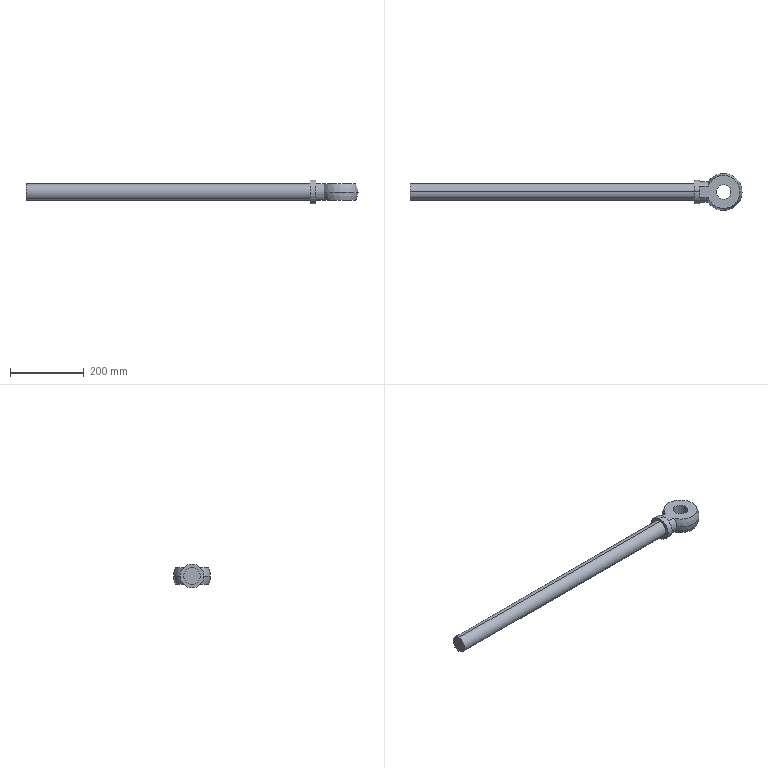Part | SolidWorks | features ICE 2, Revolution 1 | 1 solid | 15 faces | box 900 x 100 x 65 mm | volume 1587827 mm3 | cylinder 8 | plane 5 | sphere 2 | commonest cylinder face diameters 40 x2 45 x2 55 x2 65 x2
STEP:
#1=CARTESIAN_POINT('',(80.,0.,22.5));
#2=VERTEX_POINT('',#1);
#3=CARTESIAN_POINT('',(120.,0.,22.5));
#4=VERTEX_POINT('',#3);
#5=CARTESIAN_POINT('',(100.,0.,22.5));
#6=DIRECTION('',(0.,0.,1.));
#7=DIRECTION('',(1.,0.,0.));
#8=AXIS2_PLACEMENT_3D('',#5,#6,#7);
#9=CIRCLE('',#8,20.);
#10=EDGE_CURVE('',#2,#4,#9,.T.);
#11=ORIENTED_EDGE('',*,*,#10,.T.);
#12=CARTESIAN_POINT('',(120.,0.,-22.5));
#13=VERTEX_POINT('',#12);
#14=CARTESIAN_POINT('',(120.,0.,32.5));
#15=DIRECTION('',(0.,0.,-1.));
#16=VECTOR('',#15,1000.);
#17=LINE('',#14,#16);
#18=EDGE_CURVE('',#4,#13,#17,.T.);
#19=ORIENTED_EDGE('',*,*,#18,.T.);
#20=CARTESIAN_POINT('',(80.,0.,-22.5));
#21=VERTEX_POINT('',#20);
#22=CARTESIAN_POINT('',(100.,0.,-22.5));
#23=DIRECTION('',(0.,0.,-1.));
#24=DIRECTION('',(-1.,0.,0.));
#25=AXIS2_PLACEMENT_3D('',#22,#23,#24);
#26=CIRCLE('',#25,20.);
#27=EDGE_CURVE('',#13,#21,#26,.T.);
#28=ORIENTED_EDGE('',*,*,#27,.T.);
#29=CARTESIAN_POINT('',(80.,0.,32.5));
#30=DIRECTION('',(0.,0.,-1.));
#31=VECTOR('',#30,1000.);
#32=LINE('',#29,#31);
#33=EDGE_CURVE('',#2,#21,#32,.T.);
#34=ORIENTED_EDGE('',*,*,#33,.F.);
#35=EDGE_LOOP('',(#11,#19,#28,#34));
#36=FACE_OUTER_BOUND('',#35,.T.);
#37=CARTESIAN_POINT('',(100.,0.,32.5));
#38=DIRECTION('',(0.,0.,-1.));
#39=DIRECTION('',(-1.,0.,0.));
#40=AXIS2_PLACEMENT_3D('',#37,#38,#39);
#41=CYLINDRICAL_SURFACE('',#40,20.);
#42=ADVANCED_FACE('',(#36),#41,.F.);
#43=CARTESIAN_POINT('',(20.,0.,22.5));
#44=VERTEX_POINT('',#43);
#45=CARTESIAN_POINT('',(20.,0.,-22.5));
#46=VERTEX_POINT('',#45);
#47=CARTESIAN_POINT('',(20.,0.,0.));
#48=DIRECTION('',(-1.,0.,0.));
#49=DIRECTION('',(0.,0.,1.));
#50=AXIS2_PLACEMENT_3D('',#47,#48,#49);
#51=CIRCLE('',#50,22.5);
#52=EDGE_CURVE('',#44,#46,#51,.T.);
#53=ORIENTED_EDGE('',*,*,#52,.T.);
#54=CARTESIAN_POINT('',(-750.,0.,-22.5));
#55=VERTEX_POINT('',#54);
#56=CARTESIAN_POINT('',(-750.,0.,-22.5));
#57=DIRECTION('',(-1.,0.,0.));
#58=VECTOR('',#57,1000.);
#59=LINE('',#56,#58);
#60=EDGE_CURVE('',#46,#55,#59,.T.);
#61=ORIENTED_EDGE('',*,*,#60,.T.);
#62=CARTESIAN_POINT('',(-750.,0.,22.5));
#63=VERTEX_POINT('',#62);
#64=CARTESIAN_POINT('',(-750.,0.,0.));
#65=DIRECTION('',(-1.,0.,0.));
#66=DIRECTION('',(0.,0.,1.));
#67=AXIS2_PLACEMENT_3D('',#64,#65,#66);
#68=CIRCLE('',#67,22.5);
#69=EDGE_CURVE('',#63,#55,#68,.T.);
#70=ORIENTED_EDGE('',*,*,#69,.F.);
#71=CARTESIAN_POINT('',(-750.,0.,22.5));
#72=DIRECTION('',(-1.,0.,0.));
#73=VECTOR('',#72,1000.);
#74=LINE('',#71,#73);
#75=EDGE_CURVE('',#44,#63,#74,.T.);
#76=ORIENTED_EDGE('',*,*,#75,.F.);
#77=EDGE_LOOP('',(#53,#61,#70,#76));
#78=FACE_OUTER_BOUND('',#77,.T.);
#79=CARTESIAN_POINT('',(-750.,0.,0.));
#80=DIRECTION('',(-1.,0.,0.));
#81=DIRECTION('',(0.,0.,1.));
#82=AXIS2_PLACEMENT_3D('',#79,#80,#81);
#83=CYLINDRICAL_SURFACE('',#82,22.5);
#84=ADVANCED_FACE('',(#78),#83,.T.);
#85=CARTESIAN_POINT('',(35.,0.,32.5));
#86=VERTEX_POINT('',#85);
#87=CARTESIAN_POINT('',(35.,0.,-32.5));
#88=VERTEX_POINT('',#87);
#89=CARTESIAN_POINT('',(35.,0.,0.));
#90=DIRECTION('',(-1.,0.,0.));
#91=DIRECTION('',(0.,0.,1.));
#92=AXIS2_PLACEMENT_3D('',#89,#90,#91);
#93=CIRCLE('',#92,32.5);
#94=EDGE_CURVE('',#86,#88,#93,.T.);
#95=ORIENTED_EDGE('',*,*,#94,.T.);
#96=CARTESIAN_POINT('',(20.,0.,-32.5));
#97=VERTEX_POINT('',#96);
#98=CARTESIAN_POINT('',(-750.,0.,-32.5));
#99=DIRECTION('',(-1.,0.,0.));
#100=VECTOR('',#99,1000.);
#101=LINE('',#98,#100);
#102=EDGE_CURVE('',#88,#97,#101,.T.);
#103=ORIENTED_EDGE('',*,*,#102,.T.);
#104=CARTESIAN_POINT('',(20.,0.,32.5));
#105=VERTEX_POINT('',#104);
#106=CARTESIAN_POINT('',(20.,0.,0.));
#107=DIRECTION('',(-1.,0.,0.));
#108=DIRECTION('',(0.,0.,1.));
#109=AXIS2_PLACEMENT_3D('',#106,#107,#108);
#110=CIRCLE('',#109,32.5);
#111=EDGE_CURVE('',#105,#97,#110,.T.);
#112=ORIENTED_EDGE('',*,*,#111,.F.);
#113=CARTESIAN_POINT('',(-750.,0.,32.5));
#114=DIRECTION('',(-1.,0.,0.));
#115=VECTOR('',#114,1000.);
#116=LINE('',#113,#115);
#117=EDGE_CURVE('',#86,#105,#116,.T.);
#118=ORIENTED_EDGE('',*,*,#117,.F.);
#119=EDGE_LOOP('',(#95,#103,#112,#118));
#120=FACE_OUTER_BOUND('',#119,.T.);
#121=CARTESIAN_POINT('',(-750.,0.,0.));
#122=DIRECTION('',(-1.,0.,0.));
#123=DIRECTION('',(0.,0.,1.));
#124=AXIS2_PLACEMENT_3D('',#121,#122,#123);
#125=CYLINDRICAL_SURFACE('',#124,32.5);
#126=ADVANCED_FACE('',(#120),#125,.T.);
#127=CARTESIAN_POINT('',(150.,0.,0.));
#128=VERTEX_POINT('',#127);
#129=CARTESIAN_POINT('',(58.242,27.5,0.));
#130=VERTEX_POINT('',#129);
#131=CARTESIAN_POINT('',(100.,0.,0.));
#132=DIRECTION('',(0.,0.,1.));
#133=DIRECTION('',(1.,0.,0.));
#134=AXIS2_PLACEMENT_3D('',#131,#132,#133);
#135=CIRCLE('',#134,50.);
#136=EDGE_CURVE('',#128,#130,#135,.T.);
#137=ORIENTED_EDGE('',*,*,#136,.F.);
#138=CARTESIAN_POINT('',(58.242,-27.5,0.));
#139=VERTEX_POINT('',#138);
#140=CARTESIAN_POINT('',(100.,0.,0.));
#141=DIRECTION('',(0.,0.,-1.));
#142=DIRECTION('',(0.,1.,0.));
#143=AXIS2_PLACEMENT_3D('',#140,#141,#142);
#144=CIRCLE('',#143,50.);
#145=EDGE_CURVE('',#128,#139,#144,.T.);
#146=ORIENTED_EDGE('',*,*,#145,.T.);
#147=CARTESIAN_POINT('',(58.242,-15.811,-22.5));
#148=VERTEX_POINT('',#147);
#149=CARTESIAN_POINT('',(58.242,0.,0.));
#150=DIRECTION('',(-1.,0.,0.));
#151=DIRECTION('',(0.,0.,1.));
#152=AXIS2_PLACEMENT_3D('',#149,#150,#151);
#153=CIRCLE('',#152,27.5);
#154=EDGE_CURVE('',#148,#139,#153,.T.);
#155=ORIENTED_EDGE('',*,*,#154,.F.);
#156=CARTESIAN_POINT('',(58.242,15.811,-22.5));
#157=VERTEX_POINT('',#156);
#158=CARTESIAN_POINT('',(100.,0.,-22.5));
#159=DIRECTION('',(0.,0.,-1.));
#160=DIRECTION('',(-1.,0.,0.));
#161=AXIS2_PLACEMENT_3D('',#158,#159,#160);
#162=CIRCLE('',#161,44.651);
#163=EDGE_CURVE('',#157,#148,#162,.T.);
#164=ORIENTED_EDGE('',*,*,#163,.F.);
#165=CARTESIAN_POINT('',(58.242,0.,0.));
#166=DIRECTION('',(-1.,0.,0.));
#167=DIRECTION('',(0.,0.,1.));
#168=AXIS2_PLACEMENT_3D('',#165,#166,#167);
#169=CIRCLE('',#168,27.5);
#170=EDGE_CURVE('',#130,#157,#169,.T.);
#171=ORIENTED_EDGE('',*,*,#170,.F.);
#172=EDGE_LOOP('',(#137,#146,#155,#164,#171));
#173=FACE_OUTER_BOUND('',#172,.T.);
#174=CARTESIAN_POINT('',(100.,0.,0.));
#175=DIRECTION('',(0.,0.,-1.));
#176=DIRECTION('',(0.,1.,0.));
#177=AXIS2_PLACEMENT_3D('',#174,#175,#176);
#178=SPHERICAL_SURFACE('',#177,50.);
#179=ADVANCED_FACE('',(#173),#178,.T.);
#180=ORIENTED_EDGE('',*,*,#145,.F.);
#181=ORIENTED_EDGE('',*,*,#136,.T.);
#182=CARTESIAN_POINT('',(58.242,15.811,22.5));
#183=VERTEX_POINT('',#182);
#184=CARTESIAN_POINT('',(58.242,0.,0.));
#185=DIRECTION('',(-1.,0.,0.));
#186=DIRECTION('',(0.,0.,1.));
#187=AXIS2_PLACEMENT_3D('',#184,#185,#186);
#188=CIRCLE('',#187,27.5);
#189=EDGE_CURVE('',#183,#130,#188,.T.);
#190=ORIENTED_EDGE('',*,*,#189,.F.);
#191=CARTESIAN_POINT('',(58.242,-15.811,22.5));
#192=VERTEX_POINT('',#191);
#193=CARTESIAN_POINT('',(100.,0.,22.5));
#194=DIRECTION('',(0.,0.,1.));
#195=DIRECTION('',(1.,0.,0.));
#196=AXIS2_PLACEMENT_3D('',#193,#194,#195);
#197=CIRCLE('',#196,44.651);
#198=EDGE_CURVE('',#192,#183,#197,.T.);
#199=ORIENTED_EDGE('',*,*,#198,.F.);
#200=CARTESIAN_POINT('',(58.242,0.,0.));
#201=DIRECTION('',(-1.,0.,0.));
#202=DIRECTION('',(0.,0.,1.));
#203=AXIS2_PLACEMENT_3D('',#200,#201,#202);
#204=CIRCLE('',#203,27.5);
#205=EDGE_CURVE('',#139,#192,#204,.T.);
#206=ORIENTED_EDGE('',*,*,#205,.F.);
#207=EDGE_LOOP('',(#180,#181,#190,#199,#206));
#208=FACE_OUTER_BOUND('',#207,.T.);
#209=CARTESIAN_POINT('',(100.,0.,0.));
#210=DIRECTION('',(0.,0.,-1.));
#211=DIRECTION('',(0.,1.,0.));
#212=AXIS2_PLACEMENT_3D('',#209,#210,#211);
#213=SPHERICAL_SURFACE('',#212,50.);
#214=ADVANCED_FACE('',(#208),#213,.T.);
#215=CARTESIAN_POINT('',(35.,15.811,22.5));
#216=VERTEX_POINT('',#215);
#217=CARTESIAN_POINT('',(-750.,15.811,22.5));
#218=DIRECTION('',(-1.,0.,0.));
#219=VECTOR('',#218,1000.);
#220=LINE('',#217,#219);
#221=EDGE_CURVE('',#183,#216,#220,.T.);
#222=ORIENTED_EDGE('',*,*,#221,.F.);
#223=ORIENTED_EDGE('',*,*,#189,.T.);
#224=ORIENTED_EDGE('',*,*,#170,.T.);
#225=CARTESIAN_POINT('',(35.,15.811,-22.5));
#226=VERTEX_POINT('',#225);
#227=CARTESIAN_POINT('',(-750.,15.811,-22.5));
#228=DIRECTION('',(1.,0.,0.));
#229=VECTOR('',#228,1000.);
#230=LINE('',#227,#229);
#231=EDGE_CURVE('',#226,#157,#230,.T.);
#232=ORIENTED_EDGE('',*,*,#231,.F.);
#233=CARTESIAN_POINT('',(35.,0.,0.));
#234=DIRECTION('',(-1.,0.,0.));
#235=DIRECTION('',(0.,0.,1.));
#236=AXIS2_PLACEMENT_3D('',#233,#234,#235);
#237=CIRCLE('',#236,27.5);
#238=EDGE_CURVE('',#216,#226,#237,.T.);
#239=ORIENTED_EDGE('',*,*,#238,.F.);
#240=EDGE_LOOP('',(#222,#223,#224,#232,#239));
#241=FACE_OUTER_BOUND('',#240,.T.);
#242=CARTESIAN_POINT('',(-750.,0.,0.));
#243=DIRECTION('',(-1.,0.,0.));
#244=DIRECTION('',(0.,0.,1.));
#245=AXIS2_PLACEMENT_3D('',#242,#243,#244);
#246=CYLINDRICAL_SURFACE('',#245,27.5);
#247=ADVANCED_FACE('',(#241),#246,.T.);
#248=CARTESIAN_POINT('',(35.,-15.811,22.5));
#249=VERTEX_POINT('',#248);
#250=CARTESIAN_POINT('',(-750.,-15.811,22.5));
#251=DIRECTION('',(1.,0.,0.));
#252=VECTOR('',#251,1000.);
#253=LINE('',#250,#252);
#254=EDGE_CURVE('',#249,#192,#253,.T.);
#255=ORIENTED_EDGE('',*,*,#254,.F.);
#256=CARTESIAN_POINT('',(35.,-15.811,-22.5));
#257=VERTEX_POINT('',#256);
#258=CARTESIAN_POINT('',(35.,0.,0.));
#259=DIRECTION('',(-1.,0.,0.));
#260=DIRECTION('',(0.,0.,1.));
#261=AXIS2_PLACEMENT_3D('',#258,#259,#260);
#262=CIRCLE('',#261,27.5);
#263=EDGE_CURVE('',#257,#249,#262,.T.);
#264=ORIENTED_EDGE('',*,*,#263,.F.);
#265=CARTESIAN_POINT('',(-750.,-15.811,-22.5));
#266=DIRECTION('',(-1.,0.,0.));
#267=VECTOR('',#266,1000.);
#268=LINE('',#265,#267);
#269=EDGE_CURVE('',#148,#257,#268,.T.);
#270=ORIENTED_EDGE('',*,*,#269,.F.);
#271=ORIENTED_EDGE('',*,*,#154,.T.);
#272=ORIENTED_EDGE('',*,*,#205,.T.);
#273=EDGE_LOOP('',(#255,#264,#270,#271,#272));
#274=FACE_OUTER_BOUND('',#273,.T.);
#275=CARTESIAN_POINT('',(-750.,0.,0.));
#276=DIRECTION('',(-1.,0.,0.));
#277=DIRECTION('',(0.,0.,1.));
#278=AXIS2_PLACEMENT_3D('',#275,#276,#277);
#279=CYLINDRICAL_SURFACE('',#278,27.5);
#280=ADVANCED_FACE('',(#274),#279,.T.);
#281=ORIENTED_EDGE('',*,*,#263,.T.);
#282=CARTESIAN_POINT('',(35.,68.387,22.5));
#283=DIRECTION('',(0.,1.,0.));
#284=VECTOR('',#283,1000.);
#285=LINE('',#282,#284);
#286=EDGE_CURVE('',#249,#216,#285,.T.);
#287=ORIENTED_EDGE('',*,*,#286,.T.);
#288=ORIENTED_EDGE('',*,*,#238,.T.);
#289=CARTESIAN_POINT('',(35.,68.387,-22.5));
#290=DIRECTION('',(0.,-1.,0.));
#291=VECTOR('',#290,1000.);
#292=LINE('',#289,#291);
#293=EDGE_CURVE('',#226,#257,#292,.T.);
#294=ORIENTED_EDGE('',*,*,#293,.T.);
#295=EDGE_LOOP('',(#281,#287,#288,#294));
#296=FACE_BOUND('',#295,.T.);
#297=ORIENTED_EDGE('',*,*,#94,.F.);
#298=CARTESIAN_POINT('',(35.,0.,0.));
#299=DIRECTION('',(-1.,0.,0.));
#300=DIRECTION('',(0.,0.,1.));
#301=AXIS2_PLACEMENT_3D('',#298,#299,#300);
#302=CIRCLE('',#301,32.5);
#303=EDGE_CURVE('',#88,#86,#302,.T.);
#304=ORIENTED_EDGE('',*,*,#303,.F.);
#305=EDGE_LOOP('',(#297,#304));
#306=FACE_OUTER_BOUND('',#305,.T.);
#307=CARTESIAN_POINT('',(35.,32.5,0.));
#308=DIRECTION('',(-1.,0.,0.));
#309=DIRECTION('',(0.,0.,1.));
#310=AXIS2_PLACEMENT_3D('',#307,#308,#309);
#311=PLANE('',#310);
#312=ADVANCED_FACE('',(#296,#306),#311,.F.);
#313=ORIENTED_EDGE('',*,*,#102,.F.);
#314=ORIENTED_EDGE('',*,*,#303,.T.);
#315=ORIENTED_EDGE('',*,*,#117,.T.);
#316=CARTESIAN_POINT('',(20.,0.,0.));
#317=DIRECTION('',(-1.,0.,0.));
#318=DIRECTION('',(0.,0.,1.));
#319=AXIS2_PLACEMENT_3D('',#316,#317,#318);
#320=CIRCLE('',#319,32.5);
#321=EDGE_CURVE('',#97,#105,#320,.T.);
#322=ORIENTED_EDGE('',*,*,#321,.F.);
#323=EDGE_LOOP('',(#313,#314,#315,#322));
#324=FACE_OUTER_BOUND('',#323,.T.);
#325=CARTESIAN_POINT('',(-750.,0.,0.));
#326=DIRECTION('',(-1.,0.,0.));
#327=DIRECTION('',(0.,0.,1.));
#328=AXIS2_PLACEMENT_3D('',#325,#326,#327);
#329=CYLINDRICAL_SURFACE('',#328,32.5);
#330=ADVANCED_FACE('',(#324),#329,.T.);
#331=ORIENTED_EDGE('',*,*,#52,.F.);
#332=CARTESIAN_POINT('',(20.,0.,0.));
#333=DIRECTION('',(-1.,0.,0.));
#334=DIRECTION('',(0.,0.,1.));
#335=AXIS2_PLACEMENT_3D('',#332,#333,#334);
#336=CIRCLE('',#335,22.5);
#337=EDGE_CURVE('',#46,#44,#336,.T.);
#338=ORIENTED_EDGE('',*,*,#337,.F.);
#339=EDGE_LOOP('',(#331,#338));
#340=FACE_BOUND('',#339,.T.);
#341=ORIENTED_EDGE('',*,*,#111,.T.);
#342=ORIENTED_EDGE('',*,*,#321,.T.);
#343=EDGE_LOOP('',(#341,#342));
#344=FACE_OUTER_BOUND('',#343,.T.);
#345=CARTESIAN_POINT('',(20.,22.5,0.));
#346=DIRECTION('',(1.,0.,0.));
#347=DIRECTION('',(0.,0.,-1.));
#348=AXIS2_PLACEMENT_3D('',#345,#346,#347);
#349=PLANE('',#348);
#350=ADVANCED_FACE('',(#340,#344),#349,.F.);
#351=ORIENTED_EDGE('',*,*,#60,.F.);
#352=ORIENTED_EDGE('',*,*,#337,.T.);
#353=ORIENTED_EDGE('',*,*,#75,.T.);
#354=CARTESIAN_POINT('',(-750.,0.,0.));
#355=DIRECTION('',(-1.,0.,0.));
#356=DIRECTION('',(0.,0.,1.));
#357=AXIS2_PLACEMENT_3D('',#354,#355,#356);
#358=CIRCLE('',#357,22.5);
#359=EDGE_CURVE('',#55,#63,#358,.T.);
#360=ORIENTED_EDGE('',*,*,#359,.F.);
#361=EDGE_LOOP('',(#351,#352,#353,#360));
#362=FACE_OUTER_BOUND('',#361,.T.);
#363=CARTESIAN_POINT('',(-750.,0.,0.));
#364=DIRECTION('',(-1.,0.,0.));
#365=DIRECTION('',(0.,0.,1.));
#366=AXIS2_PLACEMENT_3D('',#363,#364,#365);
#367=CYLINDRICAL_SURFACE('',#366,22.5);
#368=ADVANCED_FACE('',(#362),#367,.T.);
#369=ORIENTED_EDGE('',*,*,#69,.T.);
#370=ORIENTED_EDGE('',*,*,#359,.T.);
#371=EDGE_LOOP('',(#369,#370));
#372=FACE_OUTER_BOUND('',#371,.T.);
#373=CARTESIAN_POINT('',(-750.,0.,0.));
#374=DIRECTION('',(1.,0.,0.));
#375=DIRECTION('',(0.,0.,-1.));
#376=AXIS2_PLACEMENT_3D('',#373,#374,#375);
#377=PLANE('',#376);
#378=ADVANCED_FACE('',(#372),#377,.F.);
#379=CARTESIAN_POINT('',(100.,0.,-22.5));
#380=DIRECTION('',(0.,0.,-1.));
#381=DIRECTION('',(-1.,0.,0.));
#382=AXIS2_PLACEMENT_3D('',#379,#380,#381);
#383=CIRCLE('',#382,20.);
#384=EDGE_CURVE('',#21,#13,#383,.T.);
#385=ORIENTED_EDGE('',*,*,#384,.F.);
#386=ORIENTED_EDGE('',*,*,#27,.F.);
#387=EDGE_LOOP('',(#385,#386));
#388=FACE_BOUND('',#387,.T.);
#389=ORIENTED_EDGE('',*,*,#269,.T.);
#390=ORIENTED_EDGE('',*,*,#293,.F.);
#391=ORIENTED_EDGE('',*,*,#231,.T.);
#392=ORIENTED_EDGE('',*,*,#163,.T.);
#393=EDGE_LOOP('',(#389,#390,#391,#392));
#394=FACE_OUTER_BOUND('',#393,.T.);
#395=CARTESIAN_POINT('',(150.,68.387,-22.5));
#396=DIRECTION('',(0.,0.,-1.));
#397=DIRECTION('',(-1.,0.,0.));
#398=AXIS2_PLACEMENT_3D('',#395,#396,#397);
#399=PLANE('',#398);
#400=ADVANCED_FACE('',(#388,#394),#399,.T.);
#401=ORIENTED_EDGE('',*,*,#10,.F.);
#402=CARTESIAN_POINT('',(100.,0.,22.5));
#403=DIRECTION('',(0.,0.,1.));
#404=DIRECTION('',(1.,0.,0.));
#405=AXIS2_PLACEMENT_3D('',#402,#403,#404);
#406=CIRCLE('',#405,20.);
#407=EDGE_CURVE('',#4,#2,#406,.T.);
#408=ORIENTED_EDGE('',*,*,#407,.F.);
#409=EDGE_LOOP('',(#401,#408));
#410=FACE_BOUND('',#409,.T.);
#411=ORIENTED_EDGE('',*,*,#221,.T.);
#412=ORIENTED_EDGE('',*,*,#286,.F.);
#413=ORIENTED_EDGE('',*,*,#254,.T.);
#414=ORIENTED_EDGE('',*,*,#198,.T.);
#415=EDGE_LOOP('',(#411,#412,#413,#414));
#416=FACE_OUTER_BOUND('',#415,.T.);
#417=CARTESIAN_POINT('',(150.,68.387,22.5));
#418=DIRECTION('',(0.,0.,1.));
#419=DIRECTION('',(1.,0.,0.));
#420=AXIS2_PLACEMENT_3D('',#417,#418,#419);
#421=PLANE('',#420);
#422=ADVANCED_FACE('',(#410,#416),#421,.T.);
#423=ORIENTED_EDGE('',*,*,#18,.F.);
#424=ORIENTED_EDGE('',*,*,#407,.T.);
#425=ORIENTED_EDGE('',*,*,#33,.T.);
#426=ORIENTED_EDGE('',*,*,#384,.T.);
#427=EDGE_LOOP('',(#423,#424,#425,#426));
#428=FACE_OUTER_BOUND('',#427,.T.);
#429=CARTESIAN_POINT('',(100.,0.,32.5));
#430=DIRECTION('',(0.,0.,-1.));
#431=DIRECTION('',(-1.,0.,0.));
#432=AXIS2_PLACEMENT_3D('',#429,#430,#431);
#433=CYLINDRICAL_SURFACE('',#432,20.);
#434=ADVANCED_FACE('',(#428),#433,.F.);
#435=CLOSED_SHELL('',(#42,#84,#126,#179,#214,#247,#280,#312,#330,#350,#368,#378,#400,#422,#434));
#436=MANIFOLD_SOLID_BREP('',#435);
#437=CARTESIAN_POINT('',(0.,0.,0.));
#438=DIRECTION('',(0.,0.,1.));
#439=DIRECTION('',(1.,0.,0.));
#440=AXIS2_PLACEMENT_3D('',#437,#438,#439);
#441=(LENGTH_UNIT()NAMED_UNIT(*)SI_UNIT(.MILLI.,.METRE.));
#442=UNCERTAINTY_MEASURE_WITH_UNIT(LENGTH_MEASURE(0.00001),#441,'','');
#443=(NAMED_UNIT(*)PLANE_ANGLE_UNIT()SI_UNIT($,.RADIAN.));
#444=(NAMED_UNIT(*)SI_UNIT($,.STERADIAN.)SOLID_ANGLE_UNIT());
#445=(GEOMETRIC_REPRESENTATION_CONTEXT(3)GLOBAL_UNCERTAINTY_ASSIGNED_CONTEXT((#442))GLOBAL_UNIT_ASSIGNED_CONTEXT((#441,#443,#444))REPRESENTATION_CONTEXT('',''));
#446=ADVANCED_BREP_SHAPE_REPRESENTATION('',(#436,#440),#445);